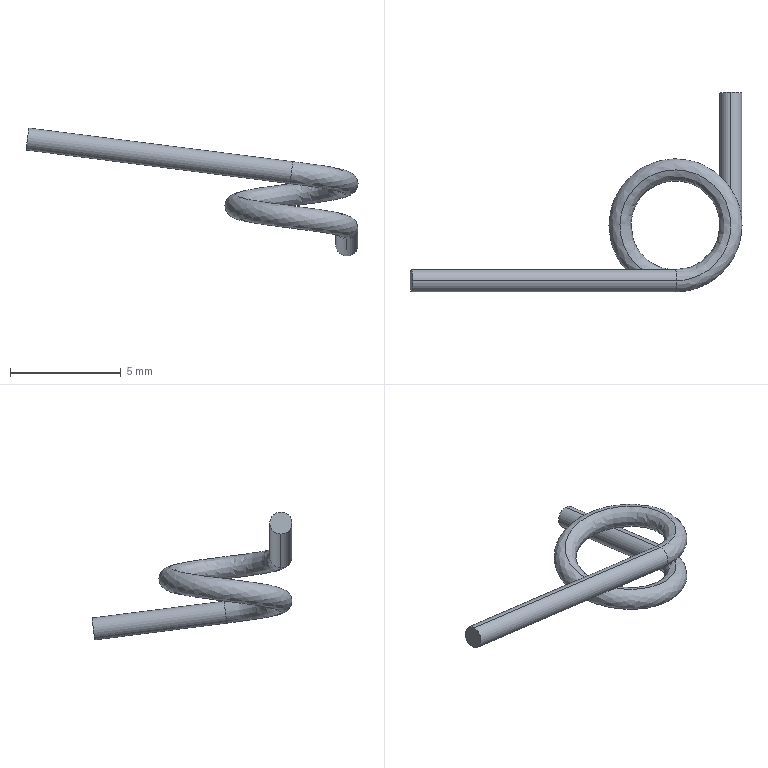Part | SolidWorks | features ICE 2, Helix 1, Sweep 1 | 1 solid | 8 faces | box 14.967 x 9.015 x 5.765 mm | volume 29.684 mm3 | cylinder 4 | spline 2 | plane 2 | commonest cylinder face diameters 1 x4
STEP:
#1=CARTESIAN_POINT('',(2.5,6.015,-0.2618));
#2=VERTEX_POINT('',#1);
#3=CARTESIAN_POINT('',(2.5,5.889,-1.254));
#4=VERTEX_POINT('',#3);
#5=CARTESIAN_POINT('',(2.5,5.952,-0.7578));
#6=DIRECTION('',(0.,0.992,-0.1263));
#7=DIRECTION('',(0.,0.1263,0.992));
#8=AXIS2_PLACEMENT_3D('',#5,#6,#7);
#9=CIRCLE('',#8,0.5);
#10=EDGE_CURVE('',#2,#4,#9,.T.);
#11=ORIENTED_EDGE('',*,*,#10,.F.);
#12=CARTESIAN_POINT('',(2.5,0.06315,0.496));
#13=VERTEX_POINT('',#12);
#14=CARTESIAN_POINT('',(2.5,6.015,-0.2618));
#15=DIRECTION('',(0.,-0.992,0.1263));
#16=VECTOR('',#15,1000.);
#17=LINE('',#14,#16);
#18=EDGE_CURVE('',#2,#13,#17,.T.);
#19=ORIENTED_EDGE('',*,*,#18,.T.);
#20=CARTESIAN_POINT('',(2.5,-0.06315,-0.496));
#21=VERTEX_POINT('',#20);
#22=CARTESIAN_POINT('',(2.5,0.,0.));
#23=DIRECTION('',(0.,-0.992,0.1263));
#24=DIRECTION('',(0.,-0.1263,-0.992));
#25=AXIS2_PLACEMENT_3D('',#22,#23,#24);
#26=CIRCLE('',#25,0.5);
#27=EDGE_CURVE('',#21,#13,#26,.T.);
#28=ORIENTED_EDGE('',*,*,#27,.F.);
#29=CARTESIAN_POINT('',(2.5,5.889,-1.254));
#30=DIRECTION('',(0.,-0.992,0.1263));
#31=VECTOR('',#30,1000.);
#32=LINE('',#29,#31);
#33=EDGE_CURVE('',#4,#21,#32,.T.);
#34=ORIENTED_EDGE('',*,*,#33,.F.);
#35=EDGE_LOOP('',(#11,#19,#28,#34));
#36=FACE_OUTER_BOUND('',#35,.T.);
#37=CARTESIAN_POINT('',(2.5,5.952,-0.7578));
#38=DIRECTION('',(0.,-0.992,0.1263));
#39=DIRECTION('',(0.,-0.1263,-0.992));
#40=AXIS2_PLACEMENT_3D('',#37,#38,#39);
#41=CYLINDRICAL_SURFACE('',#40,0.5);
#42=ADVANCED_FACE('',(#36),#41,.T.);
#43=CARTESIAN_POINT('',(-11.841,-2.5,4.512));
#44=VERTEX_POINT('',#43);
#45=CARTESIAN_POINT('',(-11.967,-2.5,3.52));
#46=VERTEX_POINT('',#45);
#47=CARTESIAN_POINT('',(-11.904,-2.5,4.016));
#48=DIRECTION('',(-0.992,0.,0.1263));
#49=DIRECTION('',(0.1263,0.,0.992));
#50=AXIS2_PLACEMENT_3D('',#47,#48,#49);
#51=CIRCLE('',#50,0.5);
#52=EDGE_CURVE('',#44,#46,#51,.T.);
#53=ORIENTED_EDGE('',*,*,#52,.F.);
#54=CARTESIAN_POINT('',(0.06315,-2.5,2.996));
#55=VERTEX_POINT('',#54);
#56=CARTESIAN_POINT('',(-11.841,-2.5,4.512));
#57=DIRECTION('',(0.992,0.,-0.1263));
#58=VECTOR('',#57,1000.);
#59=LINE('',#56,#58);
#60=EDGE_CURVE('',#44,#55,#59,.T.);
#61=ORIENTED_EDGE('',*,*,#60,.T.);
#62=CARTESIAN_POINT('',(-0.06315,-2.5,2.004));
#63=VERTEX_POINT('',#62);
#64=CARTESIAN_POINT('',(0.,-2.5,2.5));
#65=DIRECTION('',(0.992,0.,-0.1263));
#66=DIRECTION('',(-0.1263,0.,-0.992));
#67=AXIS2_PLACEMENT_3D('',#64,#65,#66);
#68=CIRCLE('',#67,0.5);
#69=EDGE_CURVE('',#63,#55,#68,.T.);
#70=ORIENTED_EDGE('',*,*,#69,.F.);
#71=CARTESIAN_POINT('',(-11.967,-2.5,3.52));
#72=DIRECTION('',(0.992,0.,-0.1263));
#73=VECTOR('',#72,1000.);
#74=LINE('',#71,#73);
#75=EDGE_CURVE('',#46,#63,#74,.T.);
#76=ORIENTED_EDGE('',*,*,#75,.F.);
#77=EDGE_LOOP('',(#53,#61,#70,#76));
#78=FACE_OUTER_BOUND('',#77,.T.);
#79=CARTESIAN_POINT('',(-11.904,-2.5,4.016));
#80=DIRECTION('',(0.992,0.,-0.1263));
#81=DIRECTION('',(-0.1263,0.,-0.992));
#82=AXIS2_PLACEMENT_3D('',#79,#80,#81);
#83=CYLINDRICAL_SURFACE('',#82,0.5);
#84=ADVANCED_FACE('',(#78),#83,.T.);
#85=ORIENTED_EDGE('',*,*,#27,.T.);
#86=CARTESIAN_POINT('',(2.5,0.06315,0.496));
#87=CARTESIAN_POINT('',(2.521,-0.7491,0.596));
#88=CARTESIAN_POINT('',(2.06,-1.418,0.696));
#89=CARTESIAN_POINT('',(1.599,-2.088,0.796));
#90=CARTESIAN_POINT('',(0.8326,-2.358,0.896));
#91=CARTESIAN_POINT('',(0.0664,-2.629,0.996));
#92=CARTESIAN_POINT('',(-0.7125,-2.397,1.096));
#93=CARTESIAN_POINT('',(-1.491,-2.166,1.196));
#94=CARTESIAN_POINT('',(-1.985,-1.521,1.296));
#95=CARTESIAN_POINT('',(-2.479,-0.8755,1.396));
#96=CARTESIAN_POINT('',(-2.5,-0.06315,1.496));
#97=CARTESIAN_POINT('',(-2.521,0.7491,1.596));
#98=CARTESIAN_POINT('',(-2.06,1.418,1.696));
#99=CARTESIAN_POINT('',(-1.599,2.088,1.796));
#100=CARTESIAN_POINT('',(-0.8326,2.358,1.896));
#101=CARTESIAN_POINT('',(-0.0664,2.629,1.996));
#102=CARTESIAN_POINT('',(0.7125,2.397,2.096));
#103=CARTESIAN_POINT('',(1.491,2.166,2.196));
#104=CARTESIAN_POINT('',(1.985,1.521,2.296));
#105=CARTESIAN_POINT('',(2.479,0.8755,2.396));
#106=CARTESIAN_POINT('',(2.5,0.06315,2.496));
#107=CARTESIAN_POINT('',(2.521,-0.7491,2.596));
#108=CARTESIAN_POINT('',(2.06,-1.418,2.696));
#109=CARTESIAN_POINT('',(1.599,-2.088,2.796));
#110=CARTESIAN_POINT('',(0.8326,-2.358,2.896));
#111=CARTESIAN_POINT('',(0.4591,-2.49,2.945));
#112=CARTESIAN_POINT('',(0.06315,-2.5,2.996));
#113=(BOUNDED_CURVE()B_SPLINE_CURVE(2,(#86,#87,#88,#89,#90,#91,#92,#93,#94,#95,#96,#97,#98,#99,#100,#101,#102,#103,#104,#105,#106,#107,#108,#109,#110,#111,#112),.UNSPECIFIED.,.F.,.F.)B_SPLINE_CURVE_WITH_KNOTS((3,2,2,2,2,2,2,2,2,2,2,2,2,3),(0.,0.05,0.1,0.15,0.2,0.25,0.3,0.35,0.4,0.45,0.5,0.55,0.6,0.625),.UNSPECIFIED.)CURVE()GEOMETRIC_REPRESENTATION_ITEM()RATIONAL_B_SPLINE_CURVE((1.,0.9511,1.,0.9511,1.,0.9511,1.,0.9511,1.,0.9511,1.,0.9511,1.,0.9511,1.,0.9511,1.,0.9511,1.,0.9511,1.,0.9511,1.,0.9511,1.,0.9755,0.9755))REPRESENTATION_ITEM(''));
#114=EDGE_CURVE('',#13,#55,#113,.T.);
#115=ORIENTED_EDGE('',*,*,#114,.T.);
#116=CARTESIAN_POINT('',(0.,-2.5,2.5));
#117=DIRECTION('',(0.992,0.,-0.1263));
#118=DIRECTION('',(-0.1263,0.,-0.992));
#119=AXIS2_PLACEMENT_3D('',#116,#117,#118);
#120=CIRCLE('',#119,0.5);
#121=EDGE_CURVE('',#55,#63,#120,.T.);
#122=ORIENTED_EDGE('',*,*,#121,.T.);
#123=CARTESIAN_POINT('',(2.5,-0.06315,-0.496));
#124=CARTESIAN_POINT('',(2.479,-0.8755,-0.396));
#125=CARTESIAN_POINT('',(1.985,-1.521,-0.296));
#126=CARTESIAN_POINT('',(1.491,-2.166,-0.196));
#127=CARTESIAN_POINT('',(0.7125,-2.397,-0.096));
#128=CARTESIAN_POINT('',(-0.0664,-2.629,0.004004));
#129=CARTESIAN_POINT('',(-0.8326,-2.358,0.104));
#130=CARTESIAN_POINT('',(-1.599,-2.088,0.204));
#131=CARTESIAN_POINT('',(-2.06,-1.418,0.304));
#132=CARTESIAN_POINT('',(-2.521,-0.7491,0.404));
#133=CARTESIAN_POINT('',(-2.5,0.06315,0.504));
#134=CARTESIAN_POINT('',(-2.479,0.8755,0.604));
#135=CARTESIAN_POINT('',(-1.985,1.521,0.704));
#136=CARTESIAN_POINT('',(-1.491,2.166,0.804));
#137=CARTESIAN_POINT('',(-0.7125,2.397,0.904));
#138=CARTESIAN_POINT('',(0.0664,2.629,1.004));
#139=CARTESIAN_POINT('',(0.8326,2.358,1.104));
#140=CARTESIAN_POINT('',(1.599,2.088,1.204));
#141=CARTESIAN_POINT('',(2.06,1.418,1.304));
#142=CARTESIAN_POINT('',(2.521,0.7491,1.404));
#143=CARTESIAN_POINT('',(2.5,-0.06315,1.504));
#144=CARTESIAN_POINT('',(2.479,-0.8755,1.604));
#145=CARTESIAN_POINT('',(1.985,-1.521,1.704));
#146=CARTESIAN_POINT('',(1.491,-2.166,1.804));
#147=CARTESIAN_POINT('',(0.7125,-2.397,1.904));
#148=CARTESIAN_POINT('',(0.3328,-2.51,1.953));
#149=CARTESIAN_POINT('',(-0.06315,-2.5,2.004));
#150=(BOUNDED_CURVE()B_SPLINE_CURVE(2,(#123,#124,#125,#126,#127,#128,#129,#130,#131,#132,#133,#134,#135,#136,#137,#138,#139,#140,#141,#142,#143,#144,#145,#146,#147,#148,#149),.UNSPECIFIED.,.F.,.F.)B_SPLINE_CURVE_WITH_KNOTS((3,2,2,2,2,2,2,2,2,2,2,2,2,3),(0.,0.05,0.1,0.15,0.2,0.25,0.3,0.35,0.4,0.45,0.5,0.55,0.6,0.625),.UNSPECIFIED.)CURVE()GEOMETRIC_REPRESENTATION_ITEM()RATIONAL_B_SPLINE_CURVE((1.,0.9511,1.,0.9511,1.,0.9511,1.,0.9511,1.,0.9511,1.,0.9511,1.,0.9511,1.,0.9511,1.,0.9511,1.,0.9511,1.,0.9511,1.,0.9511,1.,0.9755,0.9755))REPRESENTATION_ITEM(''));
#151=EDGE_CURVE('',#21,#63,#150,.T.);
#152=ORIENTED_EDGE('',*,*,#151,.F.);
#153=EDGE_LOOP('',(#85,#115,#122,#152));
#154=FACE_OUTER_BOUND('',#153,.T.);
#155=CARTESIAN_POINT('',(2.5,-0.06315,-0.496));
#156=CARTESIAN_POINT('',(2.479,-0.8755,-0.396));
#157=CARTESIAN_POINT('',(1.985,-1.521,-0.296));
#158=CARTESIAN_POINT('',(1.491,-2.166,-0.196));
#159=CARTESIAN_POINT('',(0.7125,-2.397,-0.096));
#160=CARTESIAN_POINT('',(-0.0664,-2.629,0.004004));
#161=CARTESIAN_POINT('',(-0.8326,-2.358,0.104));
#162=CARTESIAN_POINT('',(-1.599,-2.088,0.204));
#163=CARTESIAN_POINT('',(-2.06,-1.418,0.304));
#164=CARTESIAN_POINT('',(-2.521,-0.7491,0.404));
#165=CARTESIAN_POINT('',(-2.5,0.06315,0.504));
#166=CARTESIAN_POINT('',(-2.479,0.8755,0.604));
#167=CARTESIAN_POINT('',(-1.985,1.521,0.704));
#168=CARTESIAN_POINT('',(-1.491,2.166,0.804));
#169=CARTESIAN_POINT('',(-0.7125,2.397,0.904));
#170=CARTESIAN_POINT('',(0.0664,2.629,1.004));
#171=CARTESIAN_POINT('',(0.8326,2.358,1.104));
#172=CARTESIAN_POINT('',(1.599,2.088,1.204));
#173=CARTESIAN_POINT('',(2.06,1.418,1.304));
#174=CARTESIAN_POINT('',(2.521,0.7491,1.404));
#175=CARTESIAN_POINT('',(2.5,-0.06315,1.504));
#176=CARTESIAN_POINT('',(2.479,-0.8755,1.604));
#177=CARTESIAN_POINT('',(1.985,-1.521,1.704));
#178=CARTESIAN_POINT('',(1.491,-2.166,1.804));
#179=CARTESIAN_POINT('',(0.7125,-2.397,1.904));
#180=CARTESIAN_POINT('',(0.3328,-2.51,1.953));
#181=CARTESIAN_POINT('',(-0.06315,-2.5,2.004));
#182=CARTESIAN_POINT('',(3.5,-0.06315,-0.496));
#183=CARTESIAN_POINT('',(3.479,-1.2,-0.396));
#184=CARTESIAN_POINT('',(2.794,-2.108,-0.296));
#185=CARTESIAN_POINT('',(2.109,-3.016,-0.196));
#186=CARTESIAN_POINT('',(1.021,-3.348,-0.096));
#187=CARTESIAN_POINT('',(-0.0664,-3.68,0.004004));
#188=CARTESIAN_POINT('',(-1.142,-3.309,0.104));
#189=CARTESIAN_POINT('',(-2.217,-2.938,0.204));
#190=CARTESIAN_POINT('',(-2.869,-2.006,0.304));
#191=CARTESIAN_POINT('',(-3.521,-1.074,0.404));
#192=CARTESIAN_POINT('',(-3.5,0.06315,0.504));
#193=CARTESIAN_POINT('',(-3.479,1.2,0.604));
#194=CARTESIAN_POINT('',(-2.794,2.108,0.704));
#195=CARTESIAN_POINT('',(-2.109,3.016,0.804));
#196=CARTESIAN_POINT('',(-1.021,3.348,0.904));
#197=CARTESIAN_POINT('',(0.0664,3.68,1.004));
#198=CARTESIAN_POINT('',(1.142,3.309,1.104));
#199=CARTESIAN_POINT('',(2.217,2.938,1.204));
#200=CARTESIAN_POINT('',(2.869,2.006,1.304));
#201=CARTESIAN_POINT('',(3.521,1.074,1.404));
#202=CARTESIAN_POINT('',(3.5,-0.06315,1.504));
#203=CARTESIAN_POINT('',(3.479,-1.2,1.604));
#204=CARTESIAN_POINT('',(2.794,-2.108,1.704));
#205=CARTESIAN_POINT('',(2.109,-3.016,1.804));
#206=CARTESIAN_POINT('',(1.021,-3.348,1.904));
#207=CARTESIAN_POINT('',(0.4912,-3.51,1.953));
#208=CARTESIAN_POINT('',(-0.06315,-3.5,2.004));
#209=CARTESIAN_POINT('',(3.5,0.06315,0.496));
#210=CARTESIAN_POINT('',(3.521,-1.074,0.596));
#211=CARTESIAN_POINT('',(2.869,-2.006,0.696));
#212=CARTESIAN_POINT('',(2.217,-2.938,0.796));
#213=CARTESIAN_POINT('',(1.142,-3.309,0.896));
#214=CARTESIAN_POINT('',(0.0664,-3.68,0.996));
#215=CARTESIAN_POINT('',(-1.021,-3.348,1.096));
#216=CARTESIAN_POINT('',(-2.109,-3.016,1.196));
#217=CARTESIAN_POINT('',(-2.794,-2.108,1.296));
#218=CARTESIAN_POINT('',(-3.479,-1.2,1.396));
#219=CARTESIAN_POINT('',(-3.5,-0.06315,1.496));
#220=CARTESIAN_POINT('',(-3.521,1.074,1.596));
#221=CARTESIAN_POINT('',(-2.869,2.006,1.696));
#222=CARTESIAN_POINT('',(-2.217,2.938,1.796));
#223=CARTESIAN_POINT('',(-1.142,3.309,1.896));
#224=CARTESIAN_POINT('',(-0.0664,3.68,1.996));
#225=CARTESIAN_POINT('',(1.021,3.348,2.096));
#226=CARTESIAN_POINT('',(2.109,3.016,2.196));
#227=CARTESIAN_POINT('',(2.794,2.108,2.296));
#228=CARTESIAN_POINT('',(3.479,1.2,2.396));
#229=CARTESIAN_POINT('',(3.5,0.06315,2.496));
#230=CARTESIAN_POINT('',(3.521,-1.074,2.596));
#231=CARTESIAN_POINT('',(2.869,-2.006,2.696));
#232=CARTESIAN_POINT('',(2.217,-2.938,2.796));
#233=CARTESIAN_POINT('',(1.142,-3.309,2.896));
#234=CARTESIAN_POINT('',(0.6175,-3.49,2.945));
#235=CARTESIAN_POINT('',(0.06315,-3.5,2.996));
#236=CARTESIAN_POINT('',(2.5,0.06315,0.496));
#237=CARTESIAN_POINT('',(2.521,-0.7491,0.596));
#238=CARTESIAN_POINT('',(2.06,-1.418,0.696));
#239=CARTESIAN_POINT('',(1.599,-2.088,0.796));
#240=CARTESIAN_POINT('',(0.8326,-2.358,0.896));
#241=CARTESIAN_POINT('',(0.0664,-2.629,0.996));
#242=CARTESIAN_POINT('',(-0.7125,-2.397,1.096));
#243=CARTESIAN_POINT('',(-1.491,-2.166,1.196));
#244=CARTESIAN_POINT('',(-1.985,-1.521,1.296));
#245=CARTESIAN_POINT('',(-2.479,-0.8755,1.396));
#246=CARTESIAN_POINT('',(-2.5,-0.06315,1.496));
#247=CARTESIAN_POINT('',(-2.521,0.7491,1.596));
#248=CARTESIAN_POINT('',(-2.06,1.418,1.696));
#249=CARTESIAN_POINT('',(-1.599,2.088,1.796));
#250=CARTESIAN_POINT('',(-0.8326,2.358,1.896));
#251=CARTESIAN_POINT('',(-0.0664,2.629,1.996));
#252=CARTESIAN_POINT('',(0.7125,2.397,2.096));
#253=CARTESIAN_POINT('',(1.491,2.166,2.196));
#254=CARTESIAN_POINT('',(1.985,1.521,2.296));
#255=CARTESIAN_POINT('',(2.479,0.8755,2.396));
#256=CARTESIAN_POINT('',(2.5,0.06315,2.496));
#257=CARTESIAN_POINT('',(2.521,-0.7491,2.596));
#258=CARTESIAN_POINT('',(2.06,-1.418,2.696));
#259=CARTESIAN_POINT('',(1.599,-2.088,2.796));
#260=CARTESIAN_POINT('',(0.8326,-2.358,2.896));
#261=CARTESIAN_POINT('',(0.4591,-2.49,2.945));
#262=CARTESIAN_POINT('',(0.06315,-2.5,2.996));
#263=CARTESIAN_POINT('',(1.5,0.06315,0.496));
#264=CARTESIAN_POINT('',(1.521,-0.4242,0.596));
#265=CARTESIAN_POINT('',(1.251,-0.8306,0.696));
#266=CARTESIAN_POINT('',(0.9808,-1.237,0.796));
#267=CARTESIAN_POINT('',(0.5236,-1.407,0.896));
#268=CARTESIAN_POINT('',(0.0664,-1.577,0.996));
#269=CARTESIAN_POINT('',(-0.4035,-1.446,1.096));
#270=CARTESIAN_POINT('',(-0.8733,-1.315,1.196));
#271=CARTESIAN_POINT('',(-1.176,-0.9328,1.296));
#272=CARTESIAN_POINT('',(-1.479,-0.5505,1.396));
#273=CARTESIAN_POINT('',(-1.5,-0.06315,1.496));
#274=CARTESIAN_POINT('',(-1.521,0.4242,1.596));
#275=CARTESIAN_POINT('',(-1.251,0.8306,1.696));
#276=CARTESIAN_POINT('',(-0.9808,1.237,1.796));
#277=CARTESIAN_POINT('',(-0.5236,1.407,1.896));
#278=CARTESIAN_POINT('',(-0.0664,1.577,1.996));
#279=CARTESIAN_POINT('',(0.4035,1.446,2.096));
#280=CARTESIAN_POINT('',(0.8733,1.315,2.196));
#281=CARTESIAN_POINT('',(1.176,0.9328,2.296));
#282=CARTESIAN_POINT('',(1.479,0.5505,2.396));
#283=CARTESIAN_POINT('',(1.5,0.06315,2.496));
#284=CARTESIAN_POINT('',(1.521,-0.4242,2.596));
#285=CARTESIAN_POINT('',(1.251,-0.8306,2.696));
#286=CARTESIAN_POINT('',(0.9808,-1.237,2.796));
#287=CARTESIAN_POINT('',(0.5236,-1.407,2.896));
#288=CARTESIAN_POINT('',(0.3007,-1.49,2.945));
#289=CARTESIAN_POINT('',(0.06315,-1.5,2.996));
#290=CARTESIAN_POINT('',(1.5,-0.06315,-0.496));
#291=CARTESIAN_POINT('',(1.479,-0.5505,-0.396));
#292=CARTESIAN_POINT('',(1.176,-0.9328,-0.296));
#293=CARTESIAN_POINT('',(0.8733,-1.315,-0.196));
#294=CARTESIAN_POINT('',(0.4035,-1.446,-0.096));
#295=CARTESIAN_POINT('',(-0.0664,-1.577,0.004004));
#296=CARTESIAN_POINT('',(-0.5236,-1.407,0.104));
#297=CARTESIAN_POINT('',(-0.9808,-1.237,0.204));
#298=CARTESIAN_POINT('',(-1.251,-0.8306,0.304));
#299=CARTESIAN_POINT('',(-1.521,-0.4242,0.404));
#300=CARTESIAN_POINT('',(-1.5,0.06315,0.504));
#301=CARTESIAN_POINT('',(-1.479,0.5505,0.604));
#302=CARTESIAN_POINT('',(-1.176,0.9328,0.704));
#303=CARTESIAN_POINT('',(-0.8733,1.315,0.804));
#304=CARTESIAN_POINT('',(-0.4035,1.446,0.904));
#305=CARTESIAN_POINT('',(0.0664,1.577,1.004));
#306=CARTESIAN_POINT('',(0.5236,1.407,1.104));
#307=CARTESIAN_POINT('',(0.9808,1.237,1.204));
#308=CARTESIAN_POINT('',(1.251,0.8306,1.304));
#309=CARTESIAN_POINT('',(1.521,0.4242,1.404));
#310=CARTESIAN_POINT('',(1.5,-0.06315,1.504));
#311=CARTESIAN_POINT('',(1.479,-0.5505,1.604));
#312=CARTESIAN_POINT('',(1.176,-0.9328,1.704));
#313=CARTESIAN_POINT('',(0.8733,-1.315,1.804));
#314=CARTESIAN_POINT('',(0.4035,-1.446,1.904));
#315=CARTESIAN_POINT('',(0.1744,-1.51,1.953));
#316=CARTESIAN_POINT('',(-0.06315,-1.5,2.004));
#317=CARTESIAN_POINT('',(2.5,-0.06315,-0.496));
#318=CARTESIAN_POINT('',(2.479,-0.8755,-0.396));
#319=CARTESIAN_POINT('',(1.985,-1.521,-0.296));
#320=CARTESIAN_POINT('',(1.491,-2.166,-0.196));
#321=CARTESIAN_POINT('',(0.7125,-2.397,-0.096));
#322=CARTESIAN_POINT('',(-0.0664,-2.629,0.004004));
#323=CARTESIAN_POINT('',(-0.8326,-2.358,0.104));
#324=CARTESIAN_POINT('',(-1.599,-2.088,0.204));
#325=CARTESIAN_POINT('',(-2.06,-1.418,0.304));
#326=CARTESIAN_POINT('',(-2.521,-0.7491,0.404));
#327=CARTESIAN_POINT('',(-2.5,0.06315,0.504));
#328=CARTESIAN_POINT('',(-2.479,0.8755,0.604));
#329=CARTESIAN_POINT('',(-1.985,1.521,0.704));
#330=CARTESIAN_POINT('',(-1.491,2.166,0.804));
#331=CARTESIAN_POINT('',(-0.7125,2.397,0.904));
#332=CARTESIAN_POINT('',(0.0664,2.629,1.004));
#333=CARTESIAN_POINT('',(0.8326,2.358,1.104));
#334=CARTESIAN_POINT('',(1.599,2.088,1.204));
#335=CARTESIAN_POINT('',(2.06,1.418,1.304));
#336=CARTESIAN_POINT('',(2.521,0.7491,1.404));
#337=CARTESIAN_POINT('',(2.5,-0.06315,1.504));
#338=CARTESIAN_POINT('',(2.479,-0.8755,1.604));
#339=CARTESIAN_POINT('',(1.985,-1.521,1.704));
#340=CARTESIAN_POINT('',(1.491,-2.166,1.804));
#341=CARTESIAN_POINT('',(0.7125,-2.397,1.904));
#342=CARTESIAN_POINT('',(0.3328,-2.51,1.953));
#343=CARTESIAN_POINT('',(-0.06315,-2.5,2.004));
#344=(BOUNDED_SURFACE()B_SPLINE_SURFACE(3,2,((#155,#156,#157,#158,#159,#160,#161,#162,#163,#164,#165,#166,#167,#168,#169,#170,#171,#172,#173,#174,#175,#176,#177,#178,#179,#180,#181),(#182,#183,#184,#185,#186,#187,#188,#189,#190,#191,#192,#193,#194,#195,#196,#197,#198,#199,#200,#201,#202,#203,#204,#205,#206,#207,#208),(#209,#210,#211,#212,#213,#214,#215,#216,#217,#218,#219,#220,#221,#222,#223,#224,#225,#226,#227,#228,#229,#230,#231,#232,#233,#234,#235),(#236,#237,#238,#239,#240,#241,#242,#243,#244,#245,#246,#247,#248,#249,#250,#251,#252,#253,#254,#255,#256,#257,#258,#259,#260,#261,#262),(#263,#264,#265,#266,#267,#268,#269,#270,#271,#272,#273,#274,#275,#276,#277,#278,#279,#280,#281,#282,#283,#284,#285,#286,#287,#288,#289),(#290,#291,#292,#293,#294,#295,#296,#297,#298,#299,#300,#301,#302,#303,#304,#305,#306,#307,#308,#309,#310,#311,#312,#313,#314,#315,#316),(#317,#318,#319,#320,#321,#322,#323,#324,#325,#326,#327,#328,#329,#330,#331,#332,#333,#334,#335,#336,#337,#338,#339,#340,#341,#342,#343)),.UNSPECIFIED.,.T.,.F.,.F.)B_SPLINE_SURFACE_WITH_KNOTS((4,3,4),(3,2,2,2,2,2,2,2,2,2,2,2,2,3),(0.,0.5,1.),(0.,0.05,0.1,0.15,0.2,0.25,0.3,0.35,0.4,0.45,0.5,0.55,0.6,0.625),.UNSPECIFIED.)GEOMETRIC_REPRESENTATION_ITEM()RATIONAL_B_SPLINE_SURFACE(((1.,0.9511,1.,0.9511,1.,0.9511,1.,0.9511,1.,0.9511,1.,0.9511,1.,0.9511,1.,0.9511,1.,0.9511,1.,0.9511,1.,0.9511,1.,0.9511,1.,0.9755,0.9755),(0.3333,0.317,0.3333,0.317,0.3333,0.317,0.3333,0.317,0.3333,0.317,0.3333,0.317,0.3333,0.317,0.3333,0.317,0.3333,0.317,0.3333,0.317,0.3333,0.317,0.3333,0.317,0.3333,0.3252,0.3252),(0.3333,0.317,0.3333,0.317,0.3333,0.317,0.3333,0.317,0.3333,0.317,0.3333,0.317,0.3333,0.317,0.3333,0.317,0.3333,0.317,0.3333,0.317,0.3333,0.317,0.3333,0.317,0.3333,0.3252,0.3252),(1.,0.9511,1.,0.9511,1.,0.9511,1.,0.9511,1.,0.9511,1.,0.9511,1.,0.9511,1.,0.9511,1.,0.9511,1.,0.9511,1.,0.9511,1.,0.9511,1.,0.9755,0.9755),(0.3333,0.317,0.3333,0.317,0.3333,0.317,0.3333,0.317,0.3333,0.317,0.3333,0.317,0.3333,0.317,0.3333,0.317,0.3333,0.317,0.3333,0.317,0.3333,0.317,0.3333,0.317,0.3333,0.3252,0.3252),(0.3333,0.317,0.3333,0.317,0.3333,0.317,0.3333,0.317,0.3333,0.317,0.3333,0.317,0.3333,0.317,0.3333,0.317,0.3333,0.317,0.3333,0.317,0.3333,0.317,0.3333,0.317,0.3333,0.3252,0.3252),(1.,0.9511,1.,0.9511,1.,0.9511,1.,0.9511,1.,0.9511,1.,0.9511,1.,0.9511,1.,0.9511,1.,0.9511,1.,0.9511,1.,0.9511,1.,0.9511,1.,0.9755,0.9755)))REPRESENTATION_ITEM('')SURFACE());
#345=ADVANCED_FACE('',(#154),#344,.T.);
#346=ORIENTED_EDGE('',*,*,#114,.F.);
#347=CARTESIAN_POINT('',(2.5,0.,0.));
#348=DIRECTION('',(0.,-0.992,0.1263));
#349=DIRECTION('',(0.,-0.1263,-0.992));
#350=AXIS2_PLACEMENT_3D('',#347,#348,#349);
#351=CIRCLE('',#350,0.5);
#352=EDGE_CURVE('',#13,#21,#351,.T.);
#353=ORIENTED_EDGE('',*,*,#352,.T.);
#354=ORIENTED_EDGE('',*,*,#151,.T.);
#355=ORIENTED_EDGE('',*,*,#69,.T.);
#356=EDGE_LOOP('',(#346,#353,#354,#355));
#357=FACE_OUTER_BOUND('',#356,.T.);
#358=CARTESIAN_POINT('',(2.5,-0.06315,-0.496));
#359=CARTESIAN_POINT('',(2.479,-0.8755,-0.396));
#360=CARTESIAN_POINT('',(1.985,-1.521,-0.296));
#361=CARTESIAN_POINT('',(1.491,-2.166,-0.196));
#362=CARTESIAN_POINT('',(0.7125,-2.397,-0.096));
#363=CARTESIAN_POINT('',(-0.0664,-2.629,0.004004));
#364=CARTESIAN_POINT('',(-0.8326,-2.358,0.104));
#365=CARTESIAN_POINT('',(-1.599,-2.088,0.204));
#366=CARTESIAN_POINT('',(-2.06,-1.418,0.304));
#367=CARTESIAN_POINT('',(-2.521,-0.7491,0.404));
#368=CARTESIAN_POINT('',(-2.5,0.06315,0.504));
#369=CARTESIAN_POINT('',(-2.479,0.8755,0.604));
#370=CARTESIAN_POINT('',(-1.985,1.521,0.704));
#371=CARTESIAN_POINT('',(-1.491,2.166,0.804));
#372=CARTESIAN_POINT('',(-0.7125,2.397,0.904));
#373=CARTESIAN_POINT('',(0.0664,2.629,1.004));
#374=CARTESIAN_POINT('',(0.8326,2.358,1.104));
#375=CARTESIAN_POINT('',(1.599,2.088,1.204));
#376=CARTESIAN_POINT('',(2.06,1.418,1.304));
#377=CARTESIAN_POINT('',(2.521,0.7491,1.404));
#378=CARTESIAN_POINT('',(2.5,-0.06315,1.504));
#379=CARTESIAN_POINT('',(2.479,-0.8755,1.604));
#380=CARTESIAN_POINT('',(1.985,-1.521,1.704));
#381=CARTESIAN_POINT('',(1.491,-2.166,1.804));
#382=CARTESIAN_POINT('',(0.7125,-2.397,1.904));
#383=CARTESIAN_POINT('',(0.3328,-2.51,1.953));
#384=CARTESIAN_POINT('',(-0.06315,-2.5,2.004));
#385=CARTESIAN_POINT('',(3.5,-0.06315,-0.496));
#386=CARTESIAN_POINT('',(3.479,-1.2,-0.396));
#387=CARTESIAN_POINT('',(2.794,-2.108,-0.296));
#388=CARTESIAN_POINT('',(2.109,-3.016,-0.196));
#389=CARTESIAN_POINT('',(1.021,-3.348,-0.096));
#390=CARTESIAN_POINT('',(-0.0664,-3.68,0.004004));
#391=CARTESIAN_POINT('',(-1.142,-3.309,0.104));
#392=CARTESIAN_POINT('',(-2.217,-2.938,0.204));
#393=CARTESIAN_POINT('',(-2.869,-2.006,0.304));
#394=CARTESIAN_POINT('',(-3.521,-1.074,0.404));
#395=CARTESIAN_POINT('',(-3.5,0.06315,0.504));
#396=CARTESIAN_POINT('',(-3.479,1.2,0.604));
#397=CARTESIAN_POINT('',(-2.794,2.108,0.704));
#398=CARTESIAN_POINT('',(-2.109,3.016,0.804));
#399=CARTESIAN_POINT('',(-1.021,3.348,0.904));
#400=CARTESIAN_POINT('',(0.0664,3.68,1.004));
#401=CARTESIAN_POINT('',(1.142,3.309,1.104));
#402=CARTESIAN_POINT('',(2.217,2.938,1.204));
#403=CARTESIAN_POINT('',(2.869,2.006,1.304));
#404=CARTESIAN_POINT('',(3.521,1.074,1.404));
#405=CARTESIAN_POINT('',(3.5,-0.06315,1.504));
#406=CARTESIAN_POINT('',(3.479,-1.2,1.604));
#407=CARTESIAN_POINT('',(2.794,-2.108,1.704));
#408=CARTESIAN_POINT('',(2.109,-3.016,1.804));
#409=CARTESIAN_POINT('',(1.021,-3.348,1.904));
#410=CARTESIAN_POINT('',(0.4912,-3.51,1.953));
#411=CARTESIAN_POINT('',(-0.06315,-3.5,2.004));
#412=CARTESIAN_POINT('',(3.5,0.06315,0.496));
#413=CARTESIAN_POINT('',(3.521,-1.074,0.596));
#414=CARTESIAN_POINT('',(2.869,-2.006,0.696));
#415=CARTESIAN_POINT('',(2.217,-2.938,0.796));
#416=CARTESIAN_POINT('',(1.142,-3.309,0.896));
#417=CARTESIAN_POINT('',(0.0664,-3.68,0.996));
#418=CARTESIAN_POINT('',(-1.021,-3.348,1.096));
#419=CARTESIAN_POINT('',(-2.109,-3.016,1.196));
#420=CARTESIAN_POINT('',(-2.794,-2.108,1.296));
#421=CARTESIAN_POINT('',(-3.479,-1.2,1.396));
#422=CARTESIAN_POINT('',(-3.5,-0.06315,1.496));
#423=CARTESIAN_POINT('',(-3.521,1.074,1.596));
#424=CARTESIAN_POINT('',(-2.869,2.006,1.696));
#425=CARTESIAN_POINT('',(-2.217,2.938,1.796));
#426=CARTESIAN_POINT('',(-1.142,3.309,1.896));
#427=CARTESIAN_POINT('',(-0.0664,3.68,1.996));
#428=CARTESIAN_POINT('',(1.021,3.348,2.096));
#429=CARTESIAN_POINT('',(2.109,3.016,2.196));
#430=CARTESIAN_POINT('',(2.794,2.108,2.296));
#431=CARTESIAN_POINT('',(3.479,1.2,2.396));
#432=CARTESIAN_POINT('',(3.5,0.06315,2.496));
#433=CARTESIAN_POINT('',(3.521,-1.074,2.596));
#434=CARTESIAN_POINT('',(2.869,-2.006,2.696));
#435=CARTESIAN_POINT('',(2.217,-2.938,2.796));
#436=CARTESIAN_POINT('',(1.142,-3.309,2.896));
#437=CARTESIAN_POINT('',(0.6175,-3.49,2.945));
#438=CARTESIAN_POINT('',(0.06315,-3.5,2.996));
#439=CARTESIAN_POINT('',(2.5,0.06315,0.496));
#440=CARTESIAN_POINT('',(2.521,-0.7491,0.596));
#441=CARTESIAN_POINT('',(2.06,-1.418,0.696));
#442=CARTESIAN_POINT('',(1.599,-2.088,0.796));
#443=CARTESIAN_POINT('',(0.8326,-2.358,0.896));
#444=CARTESIAN_POINT('',(0.0664,-2.629,0.996));
#445=CARTESIAN_POINT('',(-0.7125,-2.397,1.096));
#446=CARTESIAN_POINT('',(-1.491,-2.166,1.196));
#447=CARTESIAN_POINT('',(-1.985,-1.521,1.296));
#448=CARTESIAN_POINT('',(-2.479,-0.8755,1.396));
#449=CARTESIAN_POINT('',(-2.5,-0.06315,1.496));
#450=CARTESIAN_POINT('',(-2.521,0.7491,1.596));
#451=CARTESIAN_POINT('',(-2.06,1.418,1.696));
#452=CARTESIAN_POINT('',(-1.599,2.088,1.796));
#453=CARTESIAN_POINT('',(-0.8326,2.358,1.896));
#454=CARTESIAN_POINT('',(-0.0664,2.629,1.996));
#455=CARTESIAN_POINT('',(0.7125,2.397,2.096));
#456=CARTESIAN_POINT('',(1.491,2.166,2.196));
#457=CARTESIAN_POINT('',(1.985,1.521,2.296));
#458=CARTESIAN_POINT('',(2.479,0.8755,2.396));
#459=CARTESIAN_POINT('',(2.5,0.06315,2.496));
#460=CARTESIAN_POINT('',(2.521,-0.7491,2.596));
#461=CARTESIAN_POINT('',(2.06,-1.418,2.696));
#462=CARTESIAN_POINT('',(1.599,-2.088,2.796));
#463=CARTESIAN_POINT('',(0.8326,-2.358,2.896));
#464=CARTESIAN_POINT('',(0.4591,-2.49,2.945));
#465=CARTESIAN_POINT('',(0.06315,-2.5,2.996));
#466=CARTESIAN_POINT('',(1.5,0.06315,0.496));
#467=CARTESIAN_POINT('',(1.521,-0.4242,0.596));
#468=CARTESIAN_POINT('',(1.251,-0.8306,0.696));
#469=CARTESIAN_POINT('',(0.9808,-1.237,0.796));
#470=CARTESIAN_POINT('',(0.5236,-1.407,0.896));
#471=CARTESIAN_POINT('',(0.0664,-1.577,0.996));
#472=CARTESIAN_POINT('',(-0.4035,-1.446,1.096));
#473=CARTESIAN_POINT('',(-0.8733,-1.315,1.196));
#474=CARTESIAN_POINT('',(-1.176,-0.9328,1.296));
#475=CARTESIAN_POINT('',(-1.479,-0.5505,1.396));
#476=CARTESIAN_POINT('',(-1.5,-0.06315,1.496));
#477=CARTESIAN_POINT('',(-1.521,0.4242,1.596));
#478=CARTESIAN_POINT('',(-1.251,0.8306,1.696));
#479=CARTESIAN_POINT('',(-0.9808,1.237,1.796));
#480=CARTESIAN_POINT('',(-0.5236,1.407,1.896));
#481=CARTESIAN_POINT('',(-0.0664,1.577,1.996));
#482=CARTESIAN_POINT('',(0.4035,1.446,2.096));
#483=CARTESIAN_POINT('',(0.8733,1.315,2.196));
#484=CARTESIAN_POINT('',(1.176,0.9328,2.296));
#485=CARTESIAN_POINT('',(1.479,0.5505,2.396));
#486=CARTESIAN_POINT('',(1.5,0.06315,2.496));
#487=CARTESIAN_POINT('',(1.521,-0.4242,2.596));
#488=CARTESIAN_POINT('',(1.251,-0.8306,2.696));
#489=CARTESIAN_POINT('',(0.9808,-1.237,2.796));
#490=CARTESIAN_POINT('',(0.5236,-1.407,2.896));
#491=CARTESIAN_POINT('',(0.3007,-1.49,2.945));
#492=CARTESIAN_POINT('',(0.06315,-1.5,2.996));
#493=CARTESIAN_POINT('',(1.5,-0.06315,-0.496));
#494=CARTESIAN_POINT('',(1.479,-0.5505,-0.396));
#495=CARTESIAN_POINT('',(1.176,-0.9328,-0.296));
#496=CARTESIAN_POINT('',(0.8733,-1.315,-0.196));
#497=CARTESIAN_POINT('',(0.4035,-1.446,-0.096));
#498=CARTESIAN_POINT('',(-0.0664,-1.577,0.004004));
#499=CARTESIAN_POINT('',(-0.5236,-1.407,0.104));
#500=CARTESIAN_POINT('',(-0.9808,-1.237,0.204));
#501=CARTESIAN_POINT('',(-1.251,-0.8306,0.304));
#502=CARTESIAN_POINT('',(-1.521,-0.4242,0.404));
#503=CARTESIAN_POINT('',(-1.5,0.06315,0.504));
#504=CARTESIAN_POINT('',(-1.479,0.5505,0.604));
#505=CARTESIAN_POINT('',(-1.176,0.9328,0.704));
#506=CARTESIAN_POINT('',(-0.8733,1.315,0.804));
#507=CARTESIAN_POINT('',(-0.4035,1.446,0.904));
#508=CARTESIAN_POINT('',(0.0664,1.577,1.004));
#509=CARTESIAN_POINT('',(0.5236,1.407,1.104));
#510=CARTESIAN_POINT('',(0.9808,1.237,1.204));
#511=CARTESIAN_POINT('',(1.251,0.8306,1.304));
#512=CARTESIAN_POINT('',(1.521,0.4242,1.404));
#513=CARTESIAN_POINT('',(1.5,-0.06315,1.504));
#514=CARTESIAN_POINT('',(1.479,-0.5505,1.604));
#515=CARTESIAN_POINT('',(1.176,-0.9328,1.704));
#516=CARTESIAN_POINT('',(0.8733,-1.315,1.804));
#517=CARTESIAN_POINT('',(0.4035,-1.446,1.904));
#518=CARTESIAN_POINT('',(0.1744,-1.51,1.953));
#519=CARTESIAN_POINT('',(-0.06315,-1.5,2.004));
#520=CARTESIAN_POINT('',(2.5,-0.06315,-0.496));
#521=CARTESIAN_POINT('',(2.479,-0.8755,-0.396));
#522=CARTESIAN_POINT('',(1.985,-1.521,-0.296));
#523=CARTESIAN_POINT('',(1.491,-2.166,-0.196));
#524=CARTESIAN_POINT('',(0.7125,-2.397,-0.096));
#525=CARTESIAN_POINT('',(-0.0664,-2.629,0.004004));
#526=CARTESIAN_POINT('',(-0.8326,-2.358,0.104));
#527=CARTESIAN_POINT('',(-1.599,-2.088,0.204));
#528=CARTESIAN_POINT('',(-2.06,-1.418,0.304));
#529=CARTESIAN_POINT('',(-2.521,-0.7491,0.404));
#530=CARTESIAN_POINT('',(-2.5,0.06315,0.504));
#531=CARTESIAN_POINT('',(-2.479,0.8755,0.604));
#532=CARTESIAN_POINT('',(-1.985,1.521,0.704));
#533=CARTESIAN_POINT('',(-1.491,2.166,0.804));
#534=CARTESIAN_POINT('',(-0.7125,2.397,0.904));
#535=CARTESIAN_POINT('',(0.0664,2.629,1.004));
#536=CARTESIAN_POINT('',(0.8326,2.358,1.104));
#537=CARTESIAN_POINT('',(1.599,2.088,1.204));
#538=CARTESIAN_POINT('',(2.06,1.418,1.304));
#539=CARTESIAN_POINT('',(2.521,0.7491,1.404));
#540=CARTESIAN_POINT('',(2.5,-0.06315,1.504));
#541=CARTESIAN_POINT('',(2.479,-0.8755,1.604));
#542=CARTESIAN_POINT('',(1.985,-1.521,1.704));
#543=CARTESIAN_POINT('',(1.491,-2.166,1.804));
#544=CARTESIAN_POINT('',(0.7125,-2.397,1.904));
#545=CARTESIAN_POINT('',(0.3328,-2.51,1.953));
#546=CARTESIAN_POINT('',(-0.06315,-2.5,2.004));
#547=(BOUNDED_SURFACE()B_SPLINE_SURFACE(3,2,((#358,#359,#360,#361,#362,#363,#364,#365,#366,#367,#368,#369,#370,#371,#372,#373,#374,#375,#376,#377,#378,#379,#380,#381,#382,#383,#384),(#385,#386,#387,#388,#389,#390,#391,#392,#393,#394,#395,#396,#397,#398,#399,#400,#401,#402,#403,#404,#405,#406,#407,#408,#409,#410,#411),(#412,#413,#414,#415,#416,#417,#418,#419,#420,#421,#422,#423,#424,#425,#426,#427,#428,#429,#430,#431,#432,#433,#434,#435,#436,#437,#438),(#439,#440,#441,#442,#443,#444,#445,#446,#447,#448,#449,#450,#451,#452,#453,#454,#455,#456,#457,#458,#459,#460,#461,#462,#463,#464,#465),(#466,#467,#468,#469,#470,#471,#472,#473,#474,#475,#476,#477,#478,#479,#480,#481,#482,#483,#484,#485,#486,#487,#488,#489,#490,#491,#492),(#493,#494,#495,#496,#497,#498,#499,#500,#501,#502,#503,#504,#505,#506,#507,#508,#509,#510,#511,#512,#513,#514,#515,#516,#517,#518,#519),(#520,#521,#522,#523,#524,#525,#526,#527,#528,#529,#530,#531,#532,#533,#534,#535,#536,#537,#538,#539,#540,#541,#542,#543,#544,#545,#546)),.UNSPECIFIED.,.T.,.F.,.F.)B_SPLINE_SURFACE_WITH_KNOTS((4,3,4),(3,2,2,2,2,2,2,2,2,2,2,2,2,3),(0.,0.5,1.),(0.,0.05,0.1,0.15,0.2,0.25,0.3,0.35,0.4,0.45,0.5,0.55,0.6,0.625),.UNSPECIFIED.)GEOMETRIC_REPRESENTATION_ITEM()RATIONAL_B_SPLINE_SURFACE(((1.,0.9511,1.,0.9511,1.,0.9511,1.,0.9511,1.,0.9511,1.,0.9511,1.,0.9511,1.,0.9511,1.,0.9511,1.,0.9511,1.,0.9511,1.,0.9511,1.,0.9755,0.9755),(0.3333,0.317,0.3333,0.317,0.3333,0.317,0.3333,0.317,0.3333,0.317,0.3333,0.317,0.3333,0.317,0.3333,0.317,0.3333,0.317,0.3333,0.317,0.3333,0.317,0.3333,0.317,0.3333,0.3252,0.3252),(0.3333,0.317,0.3333,0.317,0.3333,0.317,0.3333,0.317,0.3333,0.317,0.3333,0.317,0.3333,0.317,0.3333,0.317,0.3333,0.317,0.3333,0.317,0.3333,0.317,0.3333,0.317,0.3333,0.3252,0.3252),(1.,0.9511,1.,0.9511,1.,0.9511,1.,0.9511,1.,0.9511,1.,0.9511,1.,0.9511,1.,0.9511,1.,0.9511,1.,0.9511,1.,0.9511,1.,0.9511,1.,0.9755,0.9755),(0.3333,0.317,0.3333,0.317,0.3333,0.317,0.3333,0.317,0.3333,0.317,0.3333,0.317,0.3333,0.317,0.3333,0.317,0.3333,0.317,0.3333,0.317,0.3333,0.317,0.3333,0.317,0.3333,0.3252,0.3252),(0.3333,0.317,0.3333,0.317,0.3333,0.317,0.3333,0.317,0.3333,0.317,0.3333,0.317,0.3333,0.317,0.3333,0.317,0.3333,0.317,0.3333,0.317,0.3333,0.317,0.3333,0.317,0.3333,0.3252,0.3252),(1.,0.9511,1.,0.9511,1.,0.9511,1.,0.9511,1.,0.9511,1.,0.9511,1.,0.9511,1.,0.9511,1.,0.9511,1.,0.9511,1.,0.9511,1.,0.9511,1.,0.9755,0.9755)))REPRESENTATION_ITEM('')SURFACE());
#548=ADVANCED_FACE('',(#357),#547,.T.);
#549=ORIENTED_EDGE('',*,*,#60,.F.);
#550=CARTESIAN_POINT('',(-11.904,-2.5,4.016));
#551=DIRECTION('',(-0.992,0.,0.1263));
#552=DIRECTION('',(0.1263,0.,0.992));
#553=AXIS2_PLACEMENT_3D('',#550,#551,#552);
#554=CIRCLE('',#553,0.5);
#555=EDGE_CURVE('',#46,#44,#554,.T.);
#556=ORIENTED_EDGE('',*,*,#555,.F.);
#557=ORIENTED_EDGE('',*,*,#75,.T.);
#558=ORIENTED_EDGE('',*,*,#121,.F.);
#559=EDGE_LOOP('',(#549,#556,#557,#558));
#560=FACE_OUTER_BOUND('',#559,.T.);
#561=CARTESIAN_POINT('',(-11.904,-2.5,4.016));
#562=DIRECTION('',(0.992,0.,-0.1263));
#563=DIRECTION('',(-0.1263,0.,-0.992));
#564=AXIS2_PLACEMENT_3D('',#561,#562,#563);
#565=CYLINDRICAL_SURFACE('',#564,0.5);
#566=ADVANCED_FACE('',(#560),#565,.T.);
#567=ORIENTED_EDGE('',*,*,#555,.T.);
#568=ORIENTED_EDGE('',*,*,#52,.T.);
#569=EDGE_LOOP('',(#567,#568));
#570=FACE_OUTER_BOUND('',#569,.T.);
#571=CARTESIAN_POINT('',(-11.904,-2.5,4.016));
#572=DIRECTION('',(-0.992,0.,0.1263));
#573=DIRECTION('',(0.1263,0.,0.992));
#574=AXIS2_PLACEMENT_3D('',#571,#572,#573);
#575=PLANE('',#574);
#576=ADVANCED_FACE('',(#570),#575,.T.);
#577=ORIENTED_EDGE('',*,*,#18,.F.);
#578=CARTESIAN_POINT('',(2.5,5.952,-0.7578));
#579=DIRECTION('',(0.,0.992,-0.1263));
#580=DIRECTION('',(0.,0.1263,0.992));
#581=AXIS2_PLACEMENT_3D('',#578,#579,#580);
#582=CIRCLE('',#581,0.5);
#583=EDGE_CURVE('',#4,#2,#582,.T.);
#584=ORIENTED_EDGE('',*,*,#583,.F.);
#585=ORIENTED_EDGE('',*,*,#33,.T.);
#586=ORIENTED_EDGE('',*,*,#352,.F.);
#587=EDGE_LOOP('',(#577,#584,#585,#586));
#588=FACE_OUTER_BOUND('',#587,.T.);
#589=CARTESIAN_POINT('',(2.5,5.952,-0.7578));
#590=DIRECTION('',(0.,-0.992,0.1263));
#591=DIRECTION('',(0.,-0.1263,-0.992));
#592=AXIS2_PLACEMENT_3D('',#589,#590,#591);
#593=CYLINDRICAL_SURFACE('',#592,0.5);
#594=ADVANCED_FACE('',(#588),#593,.T.);
#595=ORIENTED_EDGE('',*,*,#583,.T.);
#596=ORIENTED_EDGE('',*,*,#10,.T.);
#597=EDGE_LOOP('',(#595,#596));
#598=FACE_OUTER_BOUND('',#597,.T.);
#599=CARTESIAN_POINT('',(2.5,5.952,-0.7578));
#600=DIRECTION('',(0.,0.992,-0.1263));
#601=DIRECTION('',(0.,0.1263,0.992));
#602=AXIS2_PLACEMENT_3D('',#599,#600,#601);
#603=PLANE('',#602);
#604=ADVANCED_FACE('',(#598),#603,.T.);
#605=CLOSED_SHELL('',(#42,#84,#345,#548,#566,#576,#594,#604));
#606=MANIFOLD_SOLID_BREP('',#605);
#607=CARTESIAN_POINT('',(0.,0.,0.));
#608=DIRECTION('',(0.,0.,1.));
#609=DIRECTION('',(1.,0.,0.));
#610=AXIS2_PLACEMENT_3D('',#607,#608,#609);
#611=(LENGTH_UNIT()NAMED_UNIT(*)SI_UNIT(.MILLI.,.METRE.));
#612=UNCERTAINTY_MEASURE_WITH_UNIT(LENGTH_MEASURE(0.00001),#611,'','');
#613=(NAMED_UNIT(*)PLANE_ANGLE_UNIT()SI_UNIT($,.RADIAN.));
#614=(NAMED_UNIT(*)SI_UNIT($,.STERADIAN.)SOLID_ANGLE_UNIT());
#615=(GEOMETRIC_REPRESENTATION_CONTEXT(3)GLOBAL_UNCERTAINTY_ASSIGNED_CONTEXT((#612))GLOBAL_UNIT_ASSIGNED_CONTEXT((#611,#613,#614))REPRESENTATION_CONTEXT('',''));
#616=ADVANCED_BREP_SHAPE_REPRESENTATION('',(#606,#610),#615);